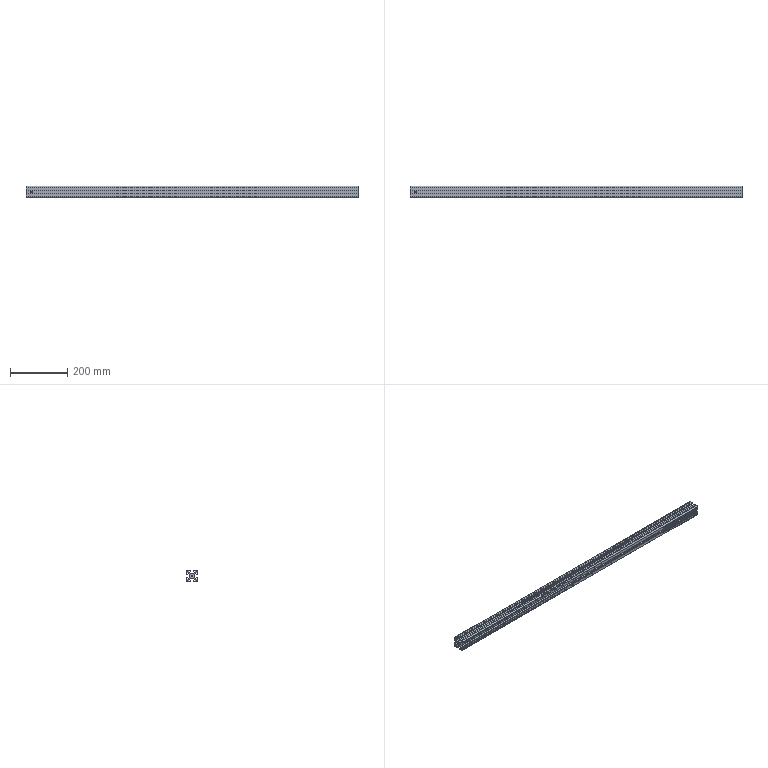Part | 1 solid | 114 faces | box 1164 x 40 x 40 mm | volume 670128 mm3 | plane 94 | cylinder 20 | commonest cylinder face diameters 8.2 x8 5 x4 6.8 x4 9 x4